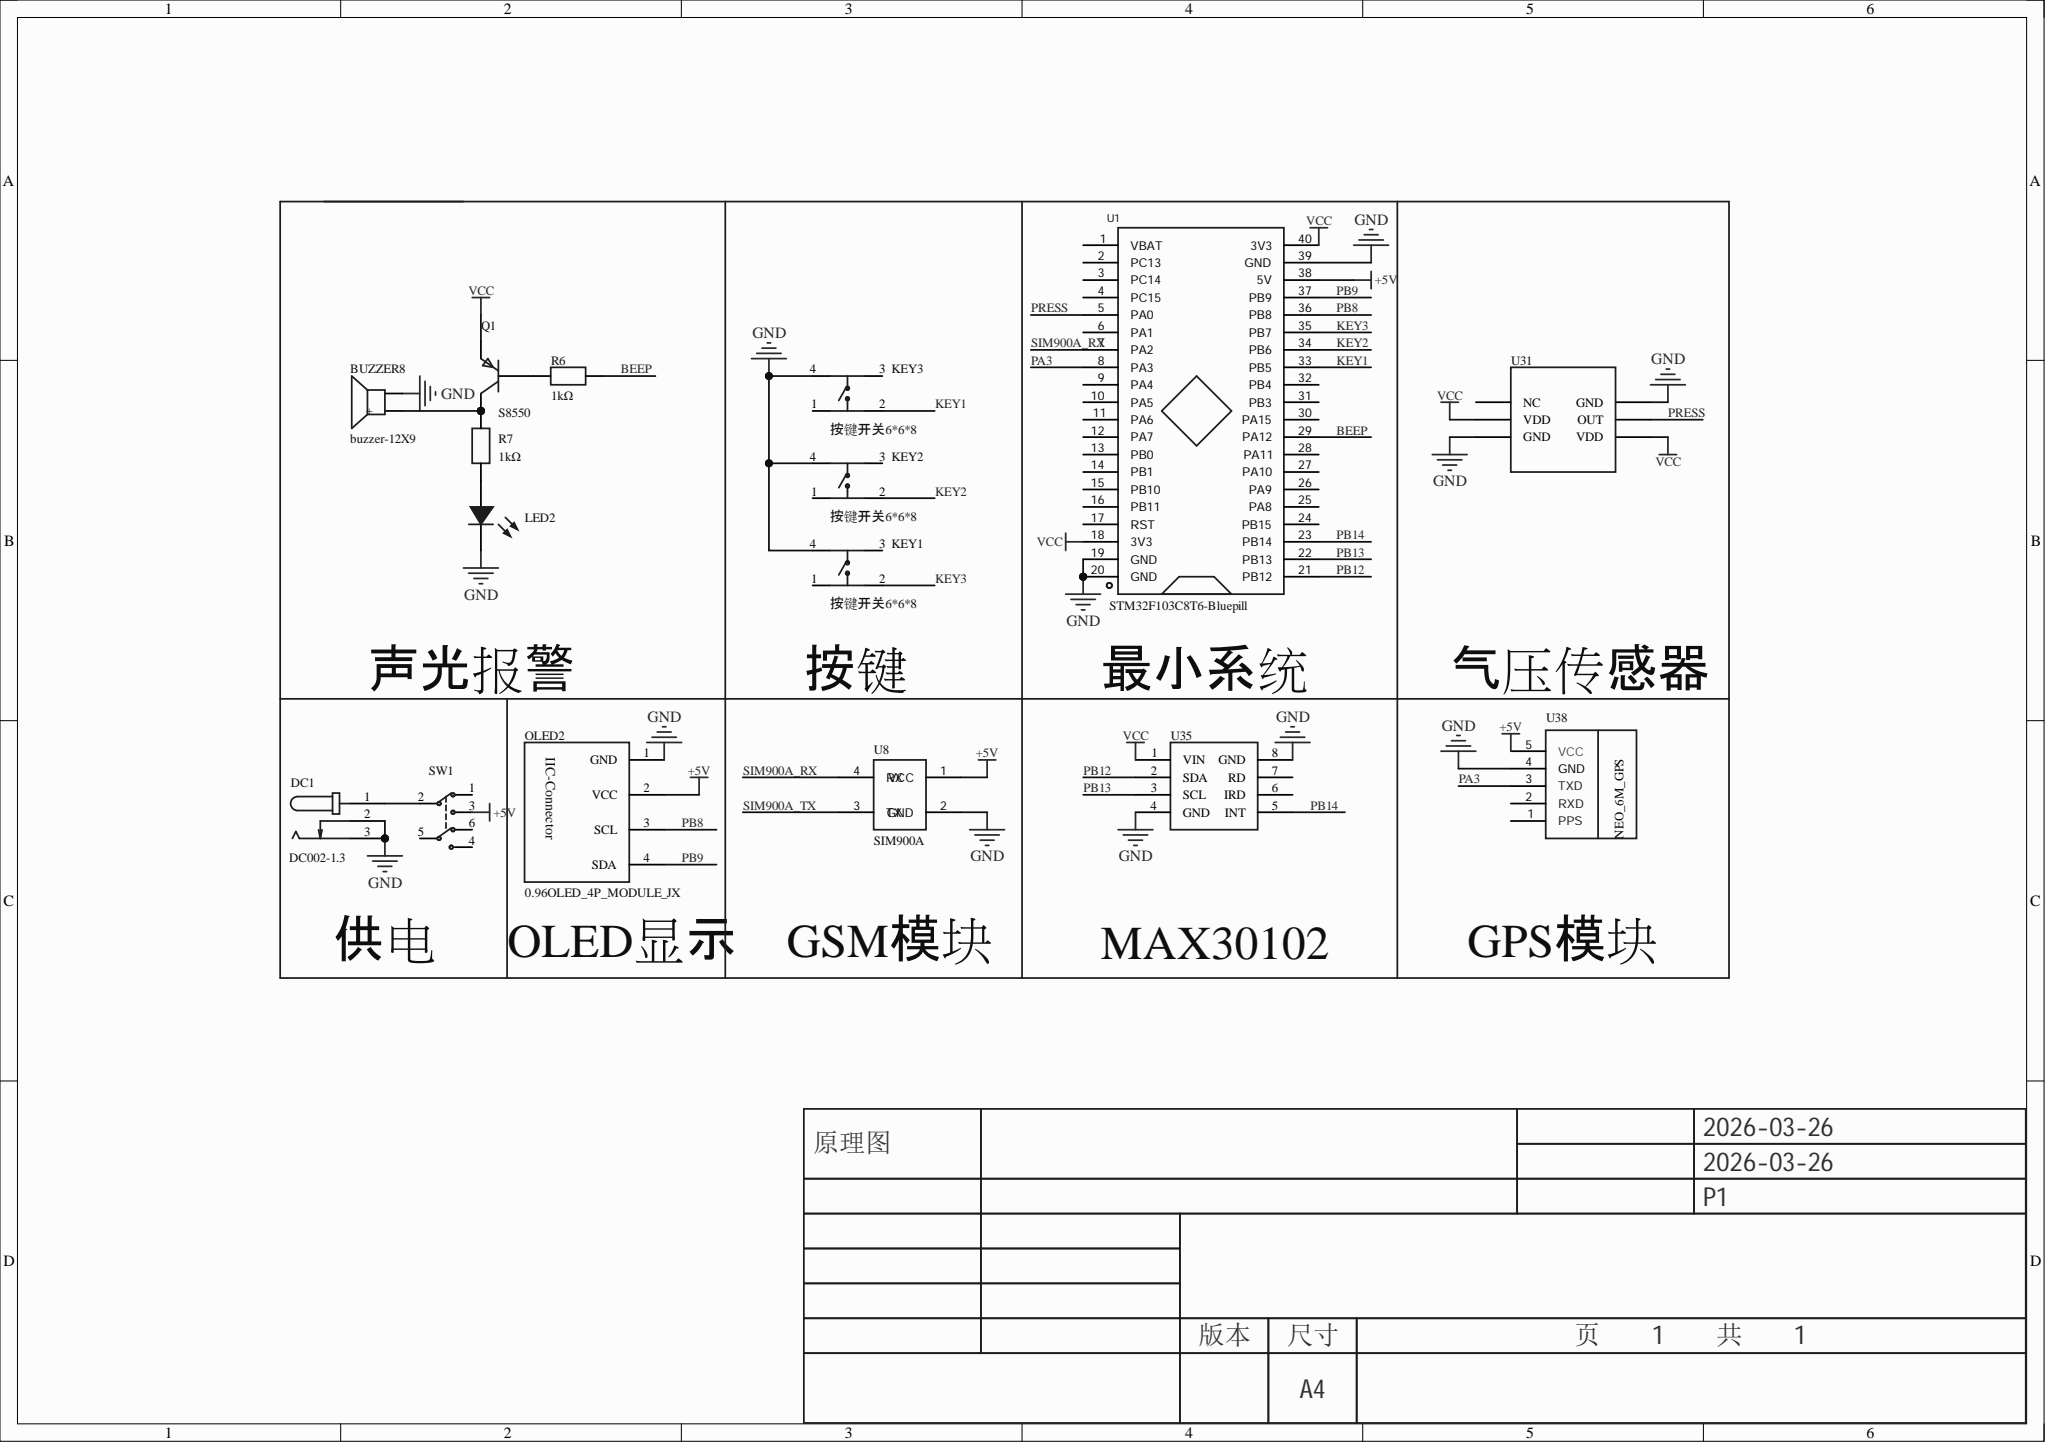Circuit board | Altium Designer | 16 parts | 19 nets
Bill of materials:
Comment,Description,Designator,Footprint,LibRef,Quantity
"buzzer-12X9","","BUZZER8","BUZ-TH_BD12.0-P7.60-D0.6-FD","buzzer-12X9","1"
"DC002-1.3","","DC1","DC-IN-TH_DC002-1.3","DC002-1.3","1"
"按键开关6*6*8","电路结构:SPST;触点额定电流:-;按钮头类型:Round Button;按钮作用方向:Top Actuated;","KEY1, KEY2, KEY3","KEY-TH_4P-L6.0-W6.0-P4.50-LS7.5","按键开关6*6*8","3"
"","","LED2","LED_TH-3mm","LED_TH-B_3mm","1"
"0.96OLED_4P_MODULE_JX","","OLED2","0.96OLED_4P","0.96OLED_4P_MODULE_JX","1"
"S8550","","Q1","TO-92-3_L4.5-W3.5-P1.27-L","S8550_C2931493","1"
"","","R6, R7","RES-TH_BD2.3-L6.5-P10.50-D0.5","插件电阻","2"
"","","SW1","自锁开关8.5*8.5","自锁开关","1"
"STM32F103C8T6-Bluepill","","U1","STM32F103C8T6-BLUEPILL","STM32F103C8T6-Bluepill","1"
"SIM900A","","U8","SIM900A","SIM900A","1"
"","","U31","AGR12 表面压力传感器","AGR12 表面压力传感器","1"
"","","U35","MAX30102","MAX30102","1"
"","GPS定位模块，串口通信","U38","NEO_6M_GPS模块","NEO_6M_GPS模块","1"
Netlist (Protel format):
[
BUZZER8
BUZ-TH_BD12.0-P7.60-D0.6-FD
buzzer-12X9



]
[
DC1
DC-IN-TH_DC002-1.3
DC002-1.3



]
[
KEY1
KEY-TH_4P-L6.0-W6.0-P4.50-LS7.5
按键开关6*6*8



]
[
KEY2
KEY-TH_4P-L6.0-W6.0-P4.50-LS7.5
按键开关6*6*8



]
[
KEY3
KEY-TH_4P-L6.0-W6.0-P4.50-LS7.5
按键开关6*6*8



]
[
LED2
LED_TH-3mm




]
[
OLED2
0.96OLED_4P
0.96OLED_4P_MODULE_JX



]
[
Q1
TO-92-3_L4.5-W3.5-P1.27-L
S8550



]
[
R6
RES-TH_BD2.3-L6.5-P10.50-D0.5




]
[
R7
RES-TH_BD2.3-L6.5-P10.50-D0.5




]
[
SW1
自锁开关8.5*8.5




]
[
U1
STM32F103C8T6-BLUEPILL
STM32F103C8T6-Bluepill



]
[
U8
SIM900A
SIM900A



]
[
U31
AGR12 表面压力传感器




]
[
U35
MAX30102




]
[
U38
NEO_6M_GPS模块




]
(
VCC
Q1-1
U1-18
U1-40
U31-2
U31-4
U35-1
)
(
SIM900A_RX
U1-7
U8-4
)
(
PRESS
U1-5
U31-5
)
(
PB14
U1-23
U35-5
)
(
PB13
U1-22
U35-3
)
(
PB12
U1-21
U35-2
)
(
PB9
OLED2-4
U1-37
)
(
PB8
OLED2-3
U1-36
)
(
PA3
U1-8
U38-3
)
(
NetQ1_2
Q1-2
R6-1
)
(
NetLED2_1
LED2-1
R7-1
)
(
NetDC1_1
DC1-1
SW1-2
)
(
NetBUZZER8_1
BUZZER8-1
Q1-3
R7-2
)
(
KEY3
KEY1-2
U1-35
)
(
KEY2
KEY2-2
U1-34
)
(
KEY1
KEY3-2
U1-33
)
(
GND
BUZZER8-2
DC1-2
DC1-3
KEY1-4
KEY2-4
KEY3-4
LED2-2
OLED2-1
U1-19
U1-20
U1-39
U8-2
U31-3
U31-6
U35-4
U35-8
U38-4
)
(
BEEP
R6-2
U1-29
)
(
+5V
OLED2-2
SW1-3
U1-38
U8-1
U38-5
)